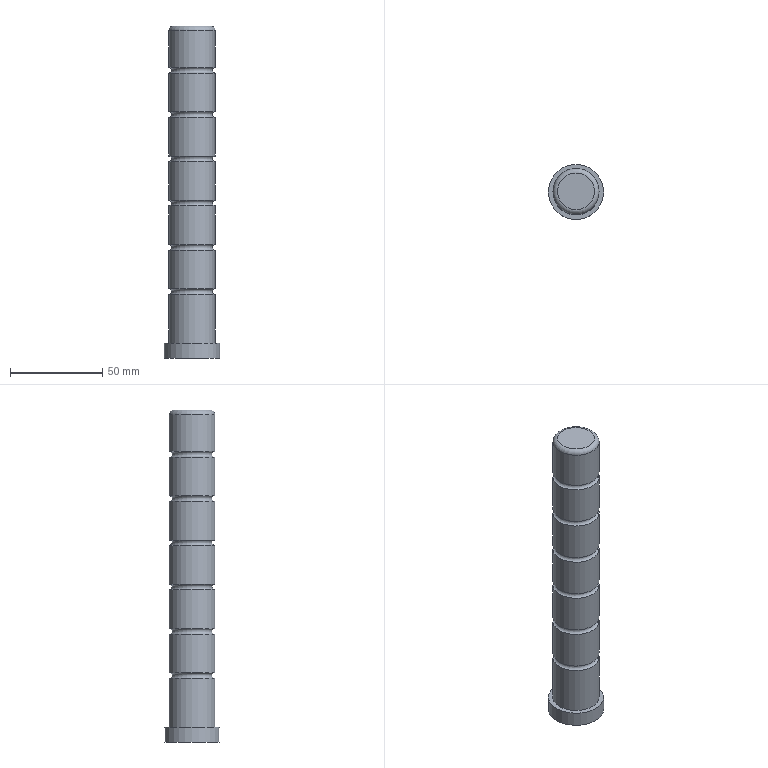Part | STEP file | solid 55 | 1 solid | 22 faces | box 30 x 30 x 180 mm | volume 84990 mm3 | cylinder 10 | torus 7 | plane 4 | cone 1 | commonest cylinder face diameters 25 x7 10.2 x1 12 x1 30 x1